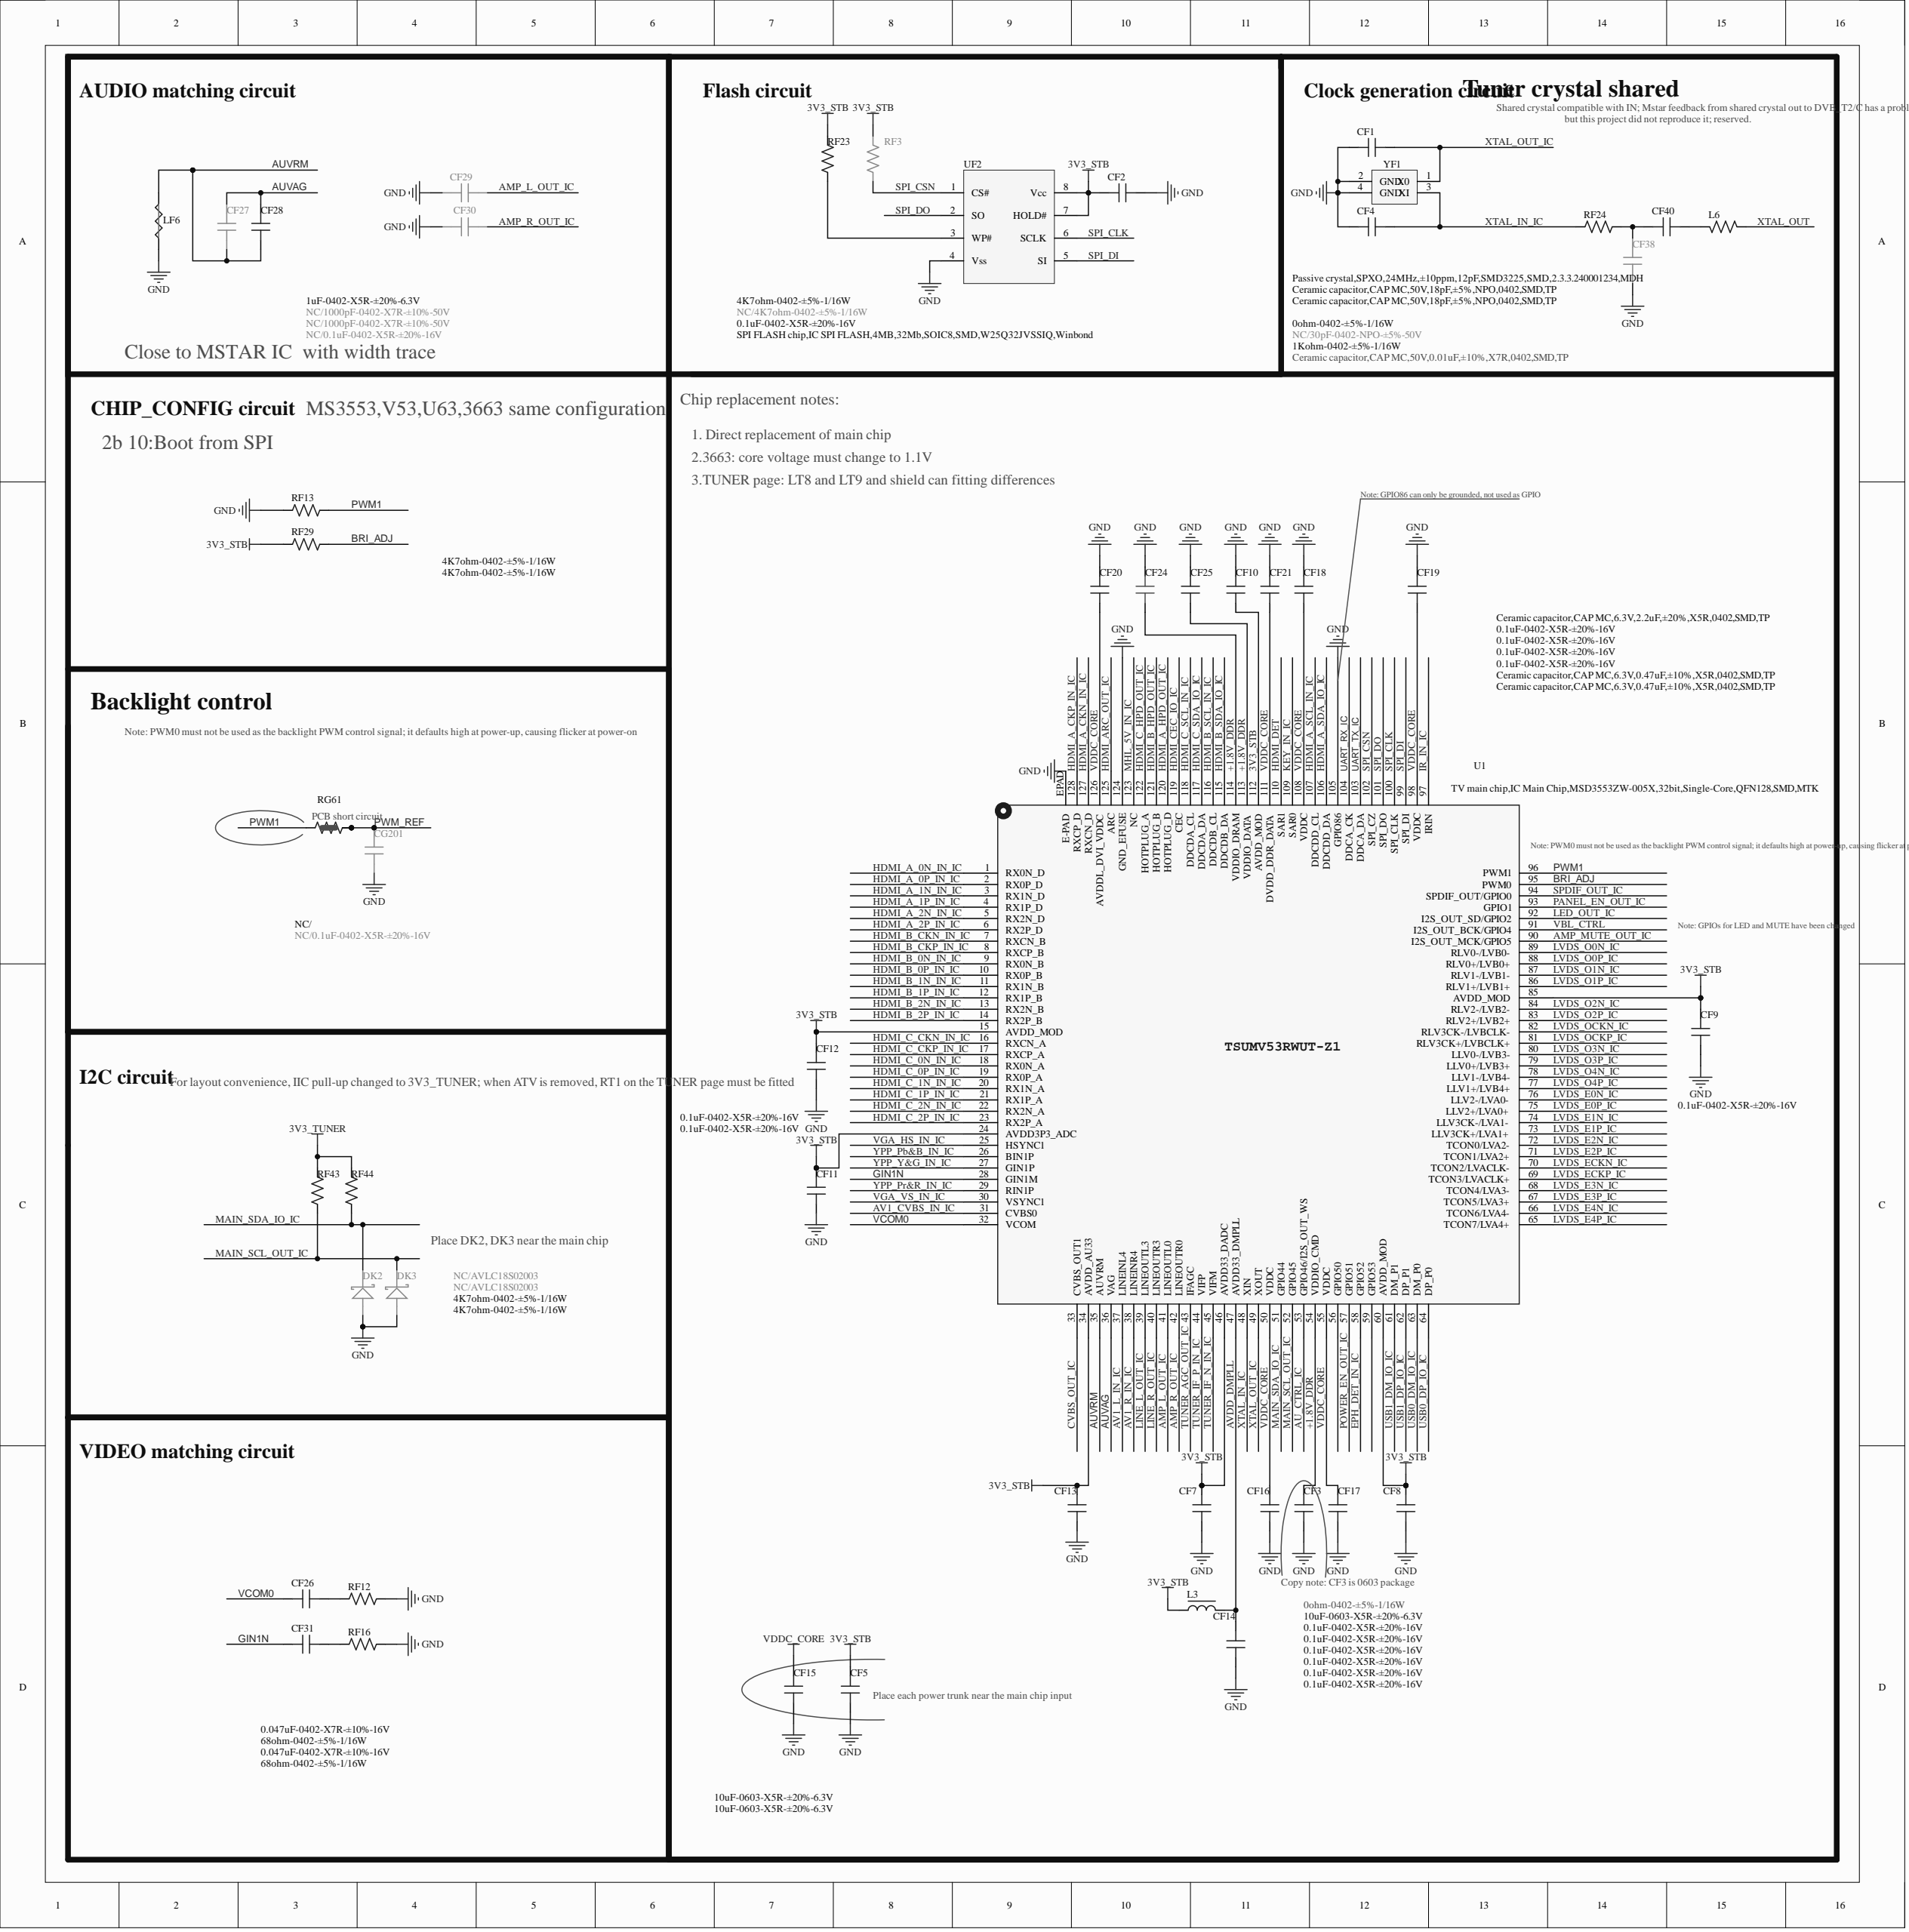Circuit board | Altium Designer | 578 parts | 300 nets | one sheet of the schematic
Parts on this sheet (reference | value | footprint):
CF1 | Ceramic capacitor,CAP MC,50V,18pF,±5%,NPO,0402,SMD,TP | C0402
CF2 | 0.1uF-0402-X5R-±20%-16V | C0402
CF3 | 10uF-0603-X5R-±20%-6.3V | C0603
CF4 | Ceramic capacitor,CAP MC,50V,18pF,±5%,NPO,0402,SMD,TP | C0402
CF5 | 10uF-0603-X5R-±20%-6.3V | C0603
CF7 | 0.1uF-0402-X5R-±20%-16V | C0402
CF8 | 0.1uF-0402-X5R-±20%-16V | C0402
CF9 | 0.1uF-0402-X5R-±20%-16V | C0402
CF10 | 0.1uF-0402-X5R-±20%-16V | C0402
CF11 | 0.1uF-0402-X5R-±20%-16V | C0402
CF12 | 0.1uF-0402-X5R-±20%-16V | C0402
CF13 | 0.1uF-0402-X5R-±20%-16V | C0402
CF14 | 0.1uF-0402-X5R-±20%-16V | C0402
CF15 | 10uF-0603-X5R-±20%-6.3V | C0603
CF16 | 0.1uF-0402-X5R-±20%-16V | C0402
CF17 | 0.1uF-0402-X5R-±20%-16V | C0402
CF18 | 0.1uF-0402-X5R-±20%-16V | C0402
CF19 | 0.1uF-0402-X5R-±20%-16V | C0402
CF20 | 0.1uF-0402-X5R-±20%-16V | C0402
CF21 | Ceramic capacitor,CAP MC,6.3V,0.47uF,±10%,X5R,0402,SMD,TP | C0402
CF24 | Ceramic capacitor,CAP MC,6.3V,2.2uF,±20%,X5R,0402,SMD,TP | C0402
CF25 | Ceramic capacitor,CAP MC,6.3V,0.47uF,±10%,X5R,0402,SMD,TP | C0402
CF26 | 0.047uF-0402-X7R-±10%-16V | C0402
CF27 | NC/0.1uF-0402-X5R-±20%-16V | C0402
CF28 | 1uF-0402-X5R-±20%-6.3V | C0402
CF29 | NC/1000pF-0402-X7R-±10%-50V | C0402
CF30 | NC/1000pF-0402-X7R-±10%-50V | C0402
CF31 | 0.047uF-0402-X7R-±10%-16V | C0402
CF38 | NC/30pF-0402-NPO-±5%-50V | C0402
CF40 | Ceramic capacitor,CAP MC,50V,0.01uF,±10%,X7R,0402,SMD,TP | C0402
CG201 | NC/0.1uF-0402-X5R-±20%-16V | C0402
DK2 | NC/AVLC18S02003 | DIODE-S0402
DK3 | NC/AVLC18S02003 | DIODE-S0402
L3 | 0ohm-0402-±5%-1/16W | L0402
L6 | 0ohm-0402-±5%-1/16W | R0402
LF6 | NC/? | GND
RF3 | NC/4K7ohm-0402-±5%-1/16W | R0402
RF12 | 68ohm-0402-±5%-1/16W | R0402
RF13 | 4K7ohm-0402-±5%-1/16W | R0402
RF16 | 68ohm-0402-±5%-1/16W | R0402
RF23 | 4K7ohm-0402-±5%-1/16W | R0402
RF24 | 1Kohm-0402-±5%-1/16W | R0402
RF29 | 4K7ohm-0402-±5%-1/16W | R0402
RF43 | 4K7ohm-0402-±5%-1/16W | R0402
RF44 | 4K7ohm-0402-±5%-1/16W | R0402
RG61 | NC/ | R0402SC
U1 | TV main chip,IC Main Chip,MSD3553ZW-005X,32bit,Single-Core,QFN128,SMD,MTK | QFN128/0.35-1-9
UF2 | SPI FLASH chip,IC SPI FLASH,4MB,32Mb,SOIC8,SMD,W25Q32JVSSIQ,Winbond | SOIC8
YF1 | Passive crystal,SPXO,24MHz,±10ppm,12pF,SMD3225,SMD,2.3.3.240001234,MDH | XTAL-S-3
Nets of these parts (net: part-pin ...):
YPP_Y&G_IN_IC: U1-27
YPP_Pr&R_IN_IC: U1-29
YPP_Pb&B_IN_IC: U1-26
XTAL_OUT_IC: CF1-2 YF1-1 U1-49
XTAL_OUT: L6-2
XTAL_IN_IC: CF4-2 RF24-2 YF1-3 U1-48
VGA_VS_IN_IC: U1-30
VGA_HS_IN_IC: U1-25
VDDC_CORE: CF15-2 CF16-2 CF17-2 CF18-1 CF19-1 CF20-2 CF21-1 U1-50 U1-55 U1-98 U1-108 U1-111 U1-126
VCOM0: CF26-1 U1-32
USB1_DP_IO_IC: U1-62
USB1_DM_IO_IC: U1-61
USB0_DP_IO_IC: U1-64
USB0_DM_IO_IC: U1-63
UART_TX_IC: U1-103
UART_RX_IC: U1-104
TUNER_IF_P_IN_IC: U1-44
TUNER_IF_N_IN_IC: U1-45
TUNER_AGC_OUT_IC: U1-43
SPI_DO: UF2-2 U1-101
SPI_DI: UF2-5 U1-99
SPI_CSN: RF3-1 UF2-1 U1-102
SPI_CLK: UF2-6 U1-100
SPDIF_OUT_IC: U1-94
PWM_REF: CG201-1 RG61-2 RG61-3
PWM1: RF13-1 RG61-1 U1-96
POWER_EN_OUT_IC: U1-57
PANEL_EN_OUT_IC: U1-93
NetRF23_1: RF23-1 UF2-3
NetCF40_1: CF40-1 L6-1
NetCF38_2: CF38-2 CF40-2 RF24-1
NetCF31_2: CF31-2 RF16-1
NetCF26_2: CF26-2 RF12-1
MAIN_SDA_IO_IC: DK2-K RF44-2 U1-51
MAIN_SCL_OUT_IC: DK3-K RF43-2 U1-52
LVDS_OCKP_IC: U1-81
LVDS_OCKN_IC: U1-82
LVDS_O3P_IC: U1-79
LVDS_O3N_IC: U1-80
LVDS_O2P_IC: U1-83
LVDS_O2N_IC: U1-84
LVDS_O1P_IC: U1-86
LVDS_O1N_IC: U1-87
LVDS_O0P_IC: U1-88
LVDS_O0N_IC: U1-89
LVDS_ECKP_IC: U1-69
LVDS_ECKN_IC: U1-70
LVDS_E3P_IC: U1-67
LVDS_E3N_IC: U1-68
LVDS_E2P_IC: U1-71
LVDS_E2N_IC: U1-72
LVDS_E1P_IC: U1-73
LVDS_E1N_IC: U1-74
LVDS_E0P_IC: U1-75
LVDS_E0N_IC: U1-76
LINE_R_OUT_IC: U1-40
LINE_L_OUT_IC: U1-39
LED_OUT_IC: U1-92
KEY_IN_IC: U1-109
IR_IN_IC: U1-97
HDMI_DET: U1-110
HDMI_CEC_IO_IC: U1-119
HDMI_B_SDA_IO_IC: U1-115
HDMI_B_SCL_IN_IC: U1-116
HDMI_B_HPD_OUT_IC: U1-121
HDMI_B_CKP_IN_IC: U1-8
HDMI_B_CKN_IN_IC: U1-7
HDMI_B_2P_IN_IC: U1-14
HDMI_B_2N_IN_IC: U1-13
HDMI_B_1P_IN_IC: U1-12
HDMI_B_1N_IN_IC: U1-11
HDMI_B_0P_IN_IC: U1-10
HDMI_B_0N_IN_IC: U1-9
HDMI_ARC_OUT_IC: U1-125
HDMI_A_SDA_IO_IC: U1-106
HDMI_A_SCL_IN_IC: U1-107
HDMI_A_HPD_OUT_IC: U1-120
HDMI_A_CKP_IN_IC: U1-128
HDMI_A_CKN_IN_IC: U1-127
HDMI_A_2P_IN_IC: U1-6
HDMI_A_2N_IN_IC: U1-5
HDMI_A_1P_IN_IC: U1-4
HDMI_A_1N_IN_IC: U1-3
HDMI_A_0P_IN_IC: U1-2
HDMI_A_0N_IN_IC: U1-1
GND: CF1-1 CF2-1 CF3-1 CF4-1 CF5-1 CF7-1 CF8-1 CF9-1 CF10-1 CF11-2 CF12-1 CF13-1 CF14-1 CF15-1 CF16-1 CF17-1 CF18-2 CF19-2 CF20-1 CF21-2 CF24-2 CF25-2 CF29-2 CF30-2 CF38-1 CG201-2 DK2-A DK3-A LF6-JP_2K RF12-2 RF13-2 RF16-2 UF2-4 YF1-2 YF1-4 U1-105 U1-124 U1-EPAD
GIN1N: CF31-1 U1-28
EPH_DET_IN_IC: U1-58
CVBS_OUT_IC: U1-33
BRI_ADJ: RF29-1 U1-95
AVDD_DMPLL: CF14-2 L3-2 U1-47
AV1_R_IN_IC: U1-38
AV1_L_IN_IC: U1-37
AV1_CVBS_IN_IC: U1-31
AUVRM: CF27-1 CF28-1 LF6-JP_1K U1-35
AUVAG: CF27-2 CF28-2 U1-36
AU_CTRL_IC: U1-53
AMP_R_OUT_IC: CF30-1 U1-42
AMP_MUTE_OUT_IC: U1-90
AMP_L_OUT_IC: CF29-1 U1-41
+1.8V_DDR: CF3-2 CF24-1 CF25-1 U1-54 U1-113 U1-114
3V3_TUNER: RF43-1 RF44-1
3V3_STB: CF2-2 CF5-2 CF7-2 CF8-2 CF9-2 CF10-2 CF11-1 CF12-2 CF13-2 L3-1 RF3-2 RF23-2 RF29-2 UF2-7 UF2-8 U1-15 U1-24 U1-34 U1-46 U1-60 U1-85 U1-112